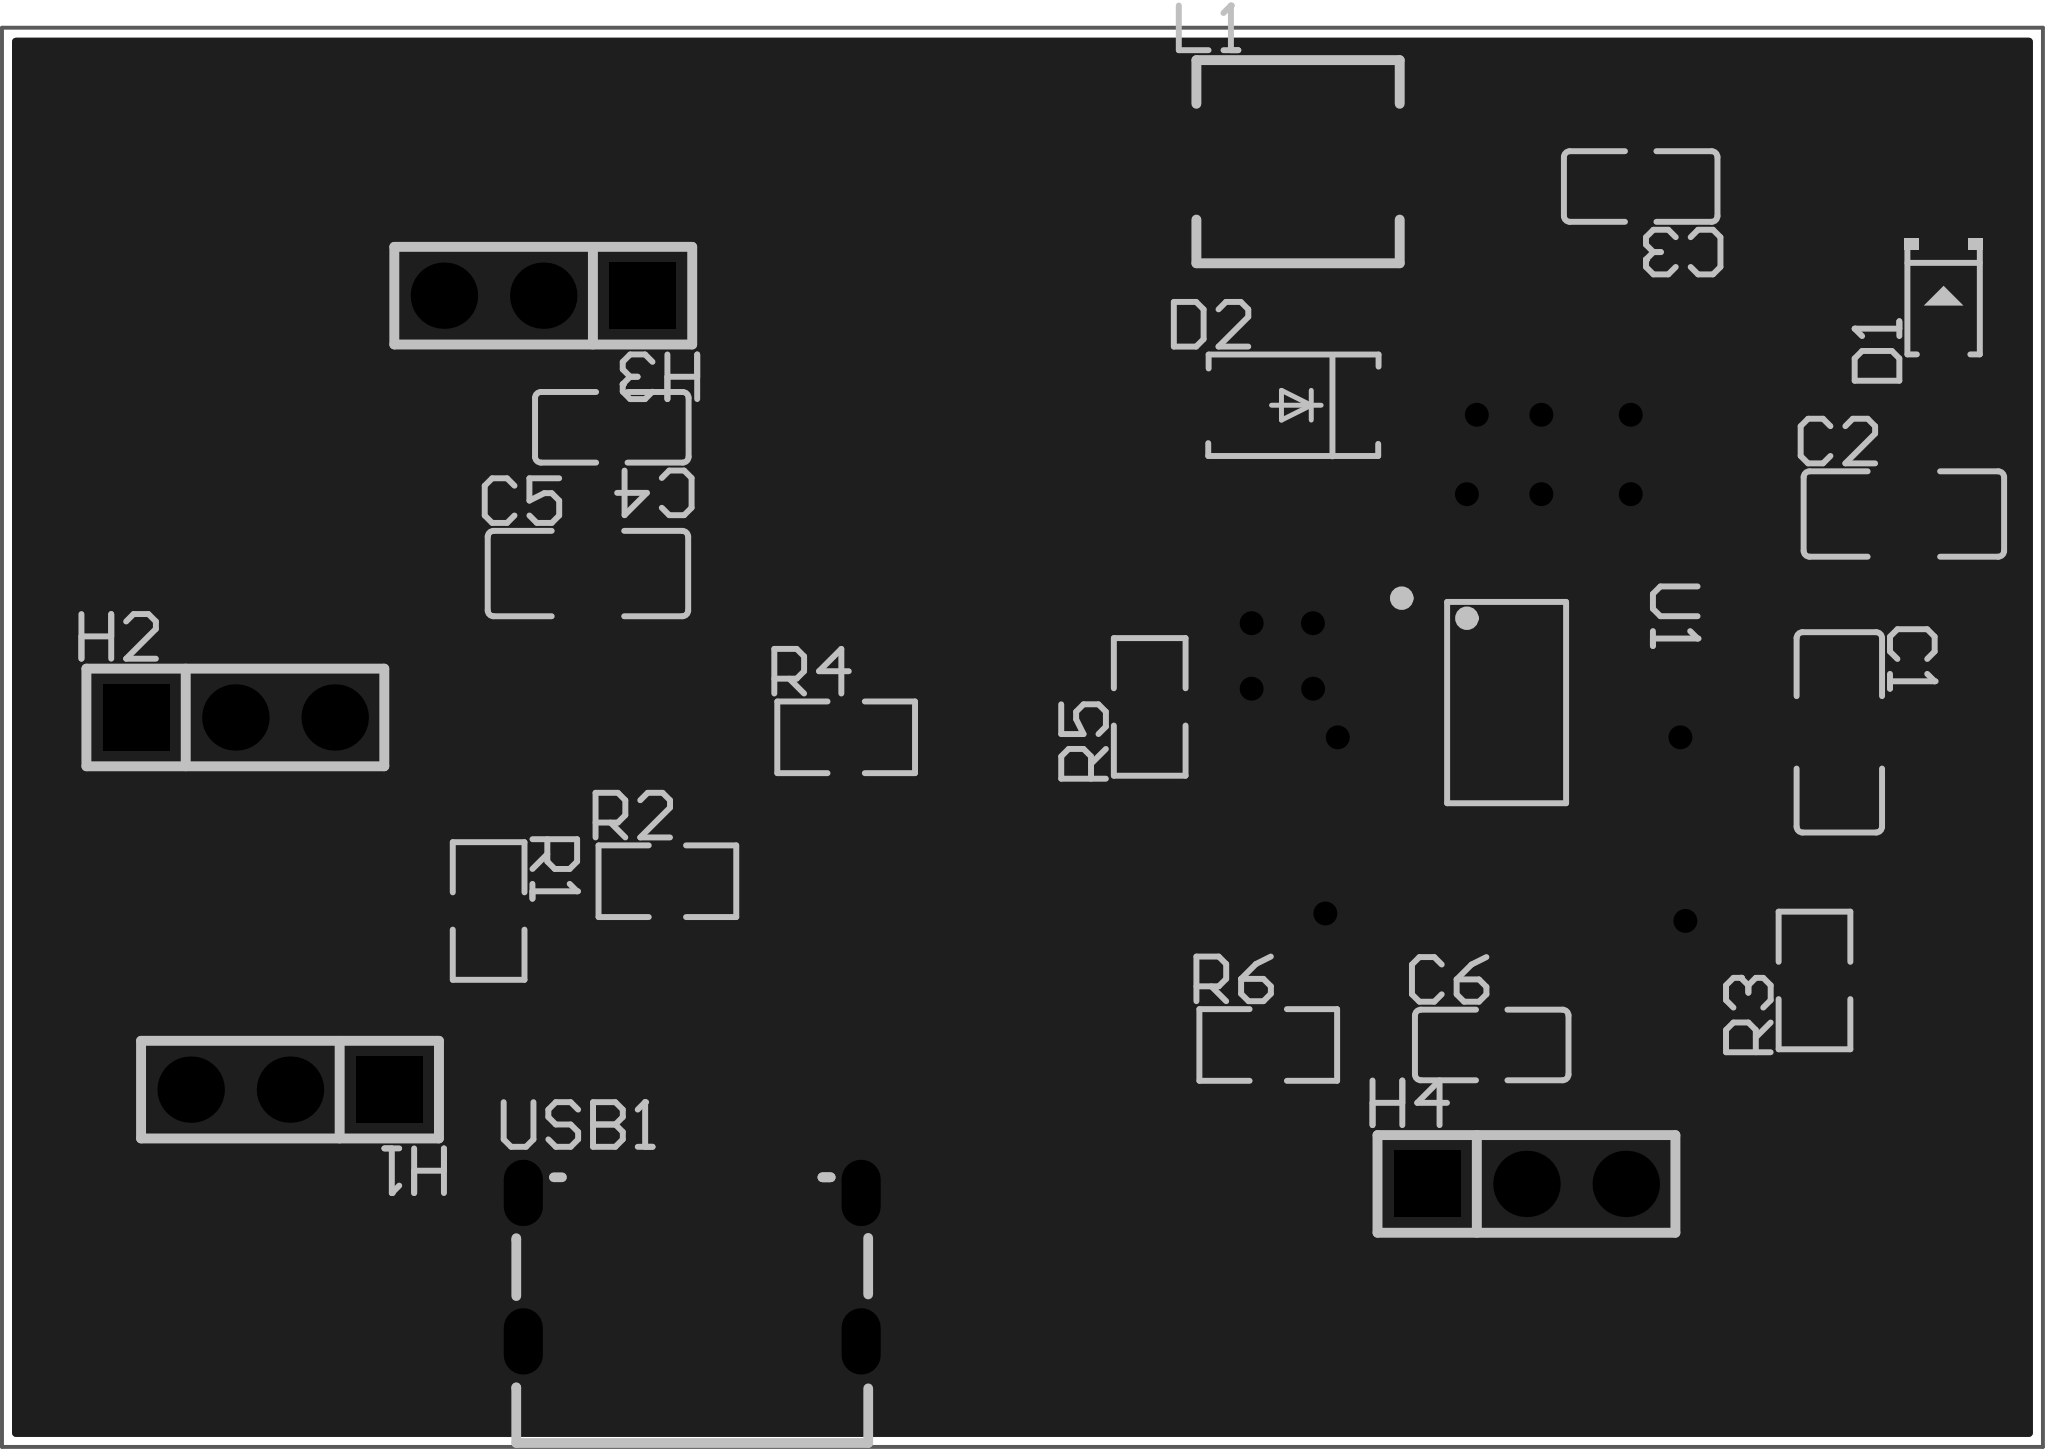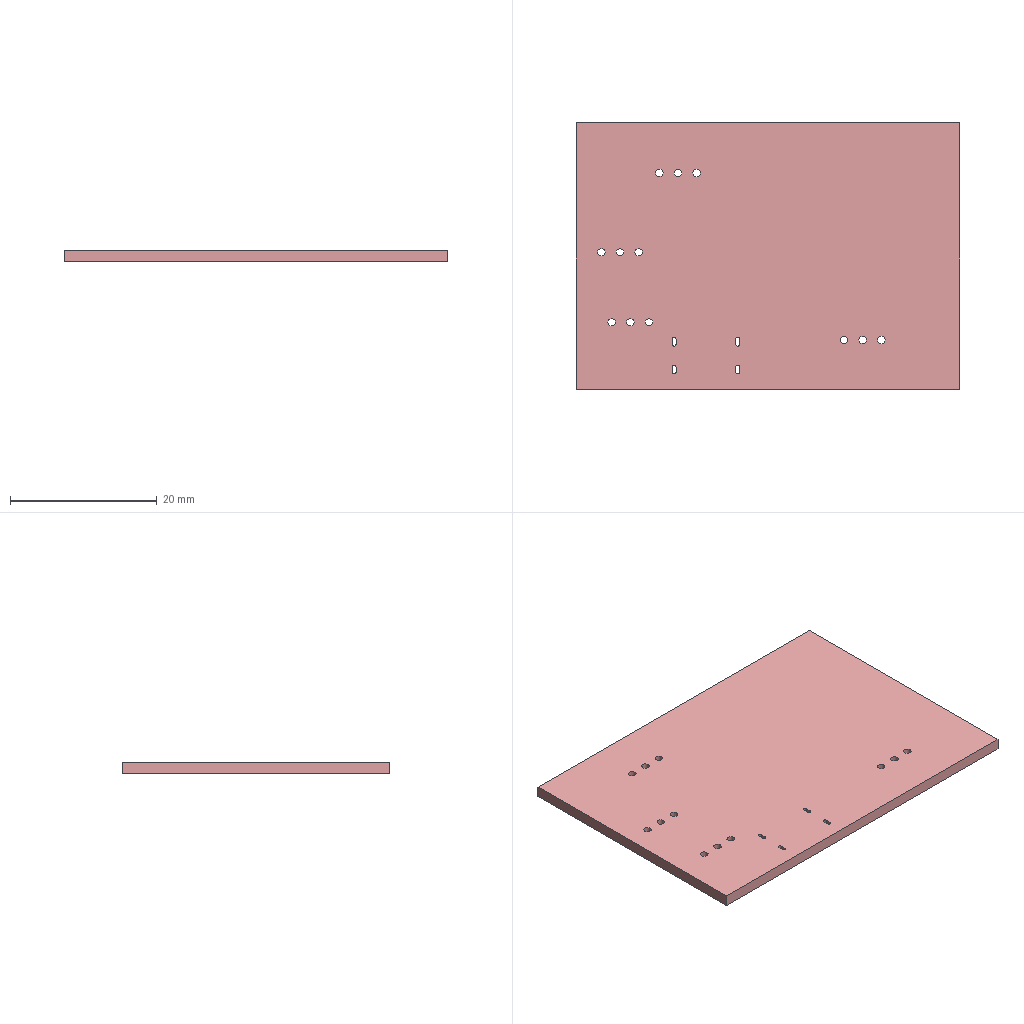Circuit board layout | Altium Designer | box 52.2 x 36.3 x 1.6 mm
Layer stack:
# Altium Designer layer stack of  (unit mm; dielectric type: 0 none, 1 core, 2 prepreg, 3 surface material)
index,name,kind,layer,copper_thickness_mm,dielectric_type,dielectric_thickness_mm,dielectric_material,dielectric_constant
0,Top Paste Mask Layer,other,,,,,,
1,Top Silkscreen Layer,other,,,,,,
2,Top Solder Mask Layer,dielectric,,,3,0.01,,3.3
3,Top Layer,copper,Top Layer,0.035,,,,
4,Dielectric1,dielectric,,,3,1.51,FR4,4.5
5,Bottom Layer,copper,Bottom Layer,0.035,,,,
6,Bottom Solder Mask Layer,dielectric,,,3,0.01,,3.3
7,Bottom Silkscreen Layer,other,,,,,,
8,Bottom Paste Mask Layer,other,,,,,,
# drill layer pairs: low layer,high layer
drill_pair,Top Layer,Bottom Layer
Part placement:
Designator,Comment,Layer,Footprint,Center-X(mm),Center-Y(mm),Rotation
C1,4.7uF,TopLayer,C1206,123.19,94.488,270
C2,4.7uF,TopLayer,C1206,124.841,100.076,0
C3,100nF,TopLayer,C0805,118.11,108.458,180
C4,100nF,TopLayer,C0805,91.797,102.295,180
C5,22uF,TopLayer,C1206,91.186,98.552,0
C6,680pF,TopLayer,C0805,114.3,86.487,0
D1,1N4148W,TopLayer,SOD-123_L2.7-W1.6-LS3.7-FD,125.857,105.537,90
D2,SS34,TopLayer,SMA_L4.3-W2.6-LS5.0-FD,109.22,102.87,0
H1,PZ254V-11-03P,TopLayer,HDR-TH_3P-P2.54-V-M_PZ254V-11-03P,83.566,85.344,180
H2,PZ254V-11-03P,TopLayer,HDR-TH_3P-P2.54-V-M_PZ254V-11-03P,82.169,94.869,0
H3,PZ254V-11-03P,TopLayer,HDR-TH_3P-P2.54-V-M_PZ254V-11-03P,90.043,105.664,180
H4,PZ254V-11-03P,TopLayer,HDR-TH_3P-P2.54-V-M_PZ254V-11-03P,115.189,82.931,0
L1,10uH,TopLayer,IND-SMD_L5.2-W5.2_MCW-0530,109.347,109.093,0
R1,5.1kΩ,TopLayer,R0805,88.646,89.916,270
R2,5.1kΩ,TopLayer,R0805,93.218,90.678,0
R3,200kΩ,TopLayer,R0805,122.555,88.138,90
R4,124kΩ,TopLayer,R0805,97.79,94.361,0
R5,40.2kΩ,TopLayer,R0805,105.553,95.139,90
R6,42.2kΩ,TopLayer,R0805,108.585,86.487,0
U1,MP4560DN-LF-Z,TopLayer,SOIC-8_L4.9-W3.9-P1.27-LS6.0-BL-EP3.1-1,114.681,95.25,270
USB1,TYPE-C 6P(073),TopLayer,TYPE-C-SMD_TYPE-C-6P-073,93.853,81.026,0
Pad and via stacks:
# Altium Designer via and pad stacks of  (unit mm). Each distinct definition once, with the count of objects using it.
# via: kind,start_layer,end_layer,hole_mm,diameter_mm,mode(0 simple;1 top-mid-bottom;2 full stack),diameter_per_layer,count,example_net
# pad: kind,layer,hole_mm,hole_type(0 round;1 square;2 slot),plating,top_size,top_shape(1 round;2 rect;3 octagon;9 rounded rect),mid_size,bottom_size,mode,footprint,size_per_layer,count,example
pad,Top Layer,0,0,plated,1.485x1.728,2,1.485x1.728,1.485x1.728,0,C1206,,6,C1.2
pad,Top Layer,0,0,plated,1.41x1.35,2,1.41x1.35,1.41x1.35,0,C0805,,6,C3.2
pad,Top Layer,0,0,plated,0.88x0.96,2,0.88x0.96,0.88x0.96,0,SOD-123_L2.7-W1.6-LS3.7-FD,,2,D1.1
pad,Top Layer,0,0,plated,1.8x1.62,2,1.8x1.62,1.8x1.62,0,SMA_L4.3-W2.6-LS5.0-FD,,2,D2.1
pad,Top Layer,0,0,plated,1.9x2.5,2,1.9x2.5,1.9x2.5,0,IND-SMD_L5.2-W5.2_MCW-0530,,2,L1.1
pad,Top Layer,0,0,plated,1.133x1.377,2,1.133x1.377,1.133x1.377,0,R0805,,12,R1.2
pad,Top Layer,0,0,plated,3.1x2.3,2,3.1x2.3,3.1x2.3,0,SOIC-8_L4.9-W3.9-P1.27-LS6.0-BL-EP3.1-1,,1,U1.9
pad,Top Layer,0,0,plated,0.63x1.865,1,0.63x1.865,0.63x1.865,0,SOIC-8_L4.9-W3.9-P1.27-LS6.0-BL-EP3.1-1,,8,U1.5
pad,Top Layer,0,0,plated,0.8x1.2,2,0.8x1.2,0.8x1.2,0,TYPE-C-SMD_TYPE-C-6P-073,,2,USB1.A12
pad,Top Layer,0,0,plated,0.7x1.2,2,0.7x1.2,0.7x1.2,0,TYPE-C-SMD_TYPE-C-6P-073,,4,USB1.A9
pad,Multi-Layer,1.02,0,plated,1.7x1.7,2,1.7x1.7,1.7x1.7,0,HDR-TH_3P-P2.54-V-M_PZ254V-11-03P,,4,H1.1
pad,Multi-Layer,1.02,0,plated,1.7x1.7,1,1.7x1.7,1.7x1.7,0,HDR-TH_3P-P2.54-V-M_PZ254V-11-03P,,8,H1.2
pad,Multi-Layer,0.5,2,plated,1x1.7,1,1x1.7,1x1.7,0,TYPE-C-SMD_TYPE-C-6P-073,,4,USB1.7
via,Top Layer,Bottom Layer,0.3048,0.61,0,,14,$1N34
Copper pours:
name,layer,net,type(0 solid;1 hatched;2 none)
Top Layer-GND,Top Layer,GND,0
Bottom Layer-GND,Bottom Layer,GND,0